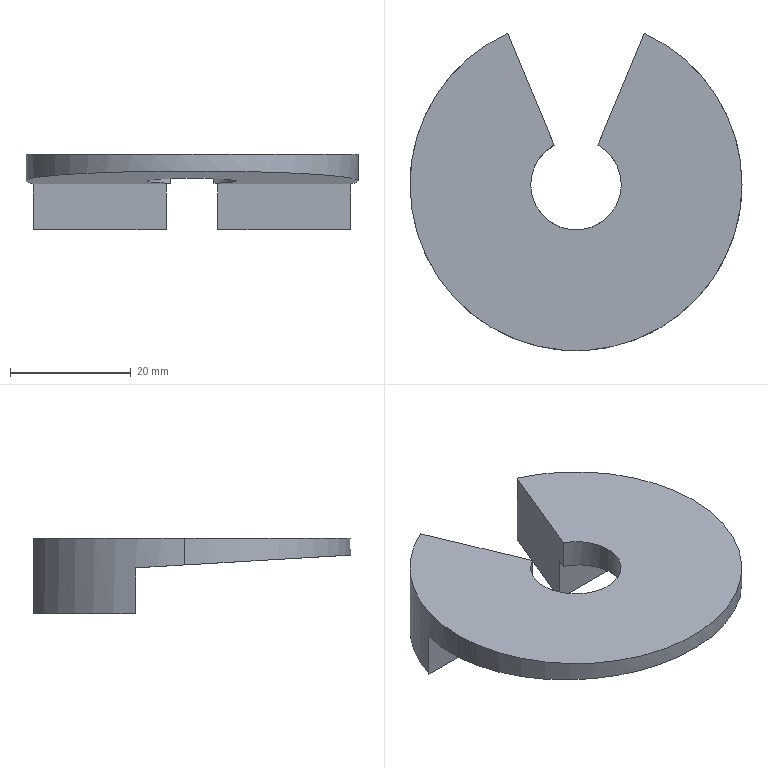Part | SolidWorks | features BaseBody 1, HoleWzd 1 | 1 solid | 22 faces | box 55 x 52.573 x 12.5 mm | volume 11112 mm3 | cylinder 10 | plane 8 | cone 4 | commonest cylinder face diameters 3.3 x4 15 x3 55 x3
STEP:
#1=CARTESIAN_POINT('',(17.65,-3.,161.));
#2=VERTEX_POINT('',#1);
#3=CARTESIAN_POINT('',(14.35,-3.,161.));
#4=VERTEX_POINT('',#3);
#5=CARTESIAN_POINT('',(16.,-3.,161.));
#6=DIRECTION('',(0.,0.,-1.));
#7=DIRECTION('',(-1.,0.,0.));
#8=AXIS2_PLACEMENT_3D('',#5,#6,#7);
#9=CIRCLE('',#8,1.65);
#10=EDGE_CURVE('',#2,#4,#9,.T.);
#11=ORIENTED_EDGE('',*,*,#10,.F.);
#12=CARTESIAN_POINT('',(17.65,-3.,154.));
#13=VERTEX_POINT('',#12);
#14=CARTESIAN_POINT('',(17.65,-3.,154.));
#15=DIRECTION('',(0.,0.,-1.));
#16=VECTOR('',#15,1000.);
#17=LINE('',#14,#16);
#18=EDGE_CURVE('',#2,#13,#17,.T.);
#19=ORIENTED_EDGE('',*,*,#18,.T.);
#20=CARTESIAN_POINT('',(14.35,-3.,154.));
#21=VERTEX_POINT('',#20);
#22=CARTESIAN_POINT('',(16.,-3.,154.));
#23=DIRECTION('',(0.,0.,-1.));
#24=DIRECTION('',(-1.,0.,0.));
#25=AXIS2_PLACEMENT_3D('',#22,#23,#24);
#26=CIRCLE('',#25,1.65);
#27=EDGE_CURVE('',#13,#21,#26,.T.);
#28=ORIENTED_EDGE('',*,*,#27,.T.);
#29=CARTESIAN_POINT('',(14.35,-3.,154.));
#30=DIRECTION('',(0.,0.,-1.));
#31=VECTOR('',#30,1000.);
#32=LINE('',#29,#31);
#33=EDGE_CURVE('',#4,#21,#32,.T.);
#34=ORIENTED_EDGE('',*,*,#33,.F.);
#35=EDGE_LOOP('',(#11,#19,#28,#34));
#36=FACE_OUTER_BOUND('',#35,.T.);
#37=CARTESIAN_POINT('',(16.,-3.,154.));
#38=DIRECTION('',(0.,0.,-1.));
#39=DIRECTION('',(-1.,0.,0.));
#40=AXIS2_PLACEMENT_3D('',#37,#38,#39);
#41=CYLINDRICAL_SURFACE('',#40,1.65);
#42=ADVANCED_FACE('',(#36),#41,.F.);
#43=CARTESIAN_POINT('',(16.,-3.,161.991));
#44=VERTEX_POINT('',#43);
#45=CARTESIAN_POINT('',(14.35,-3.,161.));
#46=DIRECTION('',(-0.8572,0.,-0.515));
#47=VECTOR('',#46,1000.);
#48=LINE('',#45,#47);
#49=EDGE_CURVE('',#44,#4,#48,.T.);
#50=ORIENTED_EDGE('',*,*,#49,.F.);
#51=CARTESIAN_POINT('',(17.65,-3.,161.));
#52=DIRECTION('',(0.8572,0.,-0.515));
#53=VECTOR('',#52,1000.);
#54=LINE('',#51,#53);
#55=EDGE_CURVE('',#44,#2,#54,.T.);
#56=ORIENTED_EDGE('',*,*,#55,.T.);
#57=ORIENTED_EDGE('',*,*,#10,.T.);
#58=EDGE_LOOP('',(#50,#56,#57));
#59=FACE_OUTER_BOUND('',#58,.T.);
#60=CARTESIAN_POINT('',(16.,-3.,161.));
#61=DIRECTION('',(0.,0.,-1.));
#62=DIRECTION('',(-1.,0.,0.));
#63=AXIS2_PLACEMENT_3D('',#60,#61,#62);
#64=CONICAL_SURFACE('',#63,1.65,1.03);
#65=ADVANCED_FACE('',(#59),#64,.F.);
#66=CARTESIAN_POINT('',(-14.35,-3.,161.));
#67=VERTEX_POINT('',#66);
#68=CARTESIAN_POINT('',(-17.65,-3.,161.));
#69=VERTEX_POINT('',#68);
#70=CARTESIAN_POINT('',(-16.,-3.,161.));
#71=DIRECTION('',(0.,0.,-1.));
#72=DIRECTION('',(-1.,0.,0.));
#73=AXIS2_PLACEMENT_3D('',#70,#71,#72);
#74=CIRCLE('',#73,1.65);
#75=EDGE_CURVE('',#67,#69,#74,.T.);
#76=ORIENTED_EDGE('',*,*,#75,.F.);
#77=CARTESIAN_POINT('',(-14.35,-3.,154.));
#78=VERTEX_POINT('',#77);
#79=CARTESIAN_POINT('',(-14.35,-3.,154.));
#80=DIRECTION('',(0.,0.,-1.));
#81=VECTOR('',#80,1000.);
#82=LINE('',#79,#81);
#83=EDGE_CURVE('',#67,#78,#82,.T.);
#84=ORIENTED_EDGE('',*,*,#83,.T.);
#85=CARTESIAN_POINT('',(-17.65,-3.,154.));
#86=VERTEX_POINT('',#85);
#87=CARTESIAN_POINT('',(-16.,-3.,154.));
#88=DIRECTION('',(0.,0.,-1.));
#89=DIRECTION('',(-1.,0.,0.));
#90=AXIS2_PLACEMENT_3D('',#87,#88,#89);
#91=CIRCLE('',#90,1.65);
#92=EDGE_CURVE('',#78,#86,#91,.T.);
#93=ORIENTED_EDGE('',*,*,#92,.T.);
#94=CARTESIAN_POINT('',(-17.65,-3.,154.));
#95=DIRECTION('',(0.,0.,-1.));
#96=VECTOR('',#95,1000.);
#97=LINE('',#94,#96);
#98=EDGE_CURVE('',#69,#86,#97,.T.);
#99=ORIENTED_EDGE('',*,*,#98,.F.);
#100=EDGE_LOOP('',(#76,#84,#93,#99));
#101=FACE_OUTER_BOUND('',#100,.T.);
#102=CARTESIAN_POINT('',(-16.,-3.,154.));
#103=DIRECTION('',(0.,0.,-1.));
#104=DIRECTION('',(-1.,0.,0.));
#105=AXIS2_PLACEMENT_3D('',#102,#103,#104);
#106=CYLINDRICAL_SURFACE('',#105,1.65);
#107=ADVANCED_FACE('',(#101),#106,.F.);
#108=CARTESIAN_POINT('',(-16.,-3.,161.991));
#109=VERTEX_POINT('',#108);
#110=CARTESIAN_POINT('',(-17.65,-3.,161.));
#111=DIRECTION('',(-0.8572,0.,-0.515));
#112=VECTOR('',#111,1000.);
#113=LINE('',#110,#112);
#114=EDGE_CURVE('',#109,#69,#113,.T.);
#115=ORIENTED_EDGE('',*,*,#114,.F.);
#116=CARTESIAN_POINT('',(-14.35,-3.,161.));
#117=DIRECTION('',(0.8572,0.,-0.515));
#118=VECTOR('',#117,1000.);
#119=LINE('',#116,#118);
#120=EDGE_CURVE('',#109,#67,#119,.T.);
#121=ORIENTED_EDGE('',*,*,#120,.T.);
#122=ORIENTED_EDGE('',*,*,#75,.T.);
#123=EDGE_LOOP('',(#115,#121,#122));
#124=FACE_OUTER_BOUND('',#123,.T.);
#125=CARTESIAN_POINT('',(-16.,-3.,161.));
#126=DIRECTION('',(0.,0.,-1.));
#127=DIRECTION('',(-1.,0.,0.));
#128=AXIS2_PLACEMENT_3D('',#125,#126,#127);
#129=CONICAL_SURFACE('',#128,1.65,1.03);
#130=ADVANCED_FACE('',(#124),#129,.F.);
#131=CARTESIAN_POINT('',(7.5,-17.,166.5));
#132=VERTEX_POINT('',#131);
#133=CARTESIAN_POINT('',(-7.5,-17.,166.5));
#134=VERTEX_POINT('',#133);
#135=CARTESIAN_POINT('',(0.,-17.,166.5));
#136=DIRECTION('',(0.,0.,-1.));
#137=DIRECTION('',(-1.,0.,0.));
#138=AXIS2_PLACEMENT_3D('',#135,#136,#137);
#139=CIRCLE('',#138,7.5);
#140=EDGE_CURVE('',#132,#134,#139,.T.);
#141=ORIENTED_EDGE('',*,*,#140,.F.);
#142=CARTESIAN_POINT('',(7.5,-17.,162.084));
#143=VERTEX_POINT('',#142);
#144=CARTESIAN_POINT('',(7.5,-17.,166.5));
#145=DIRECTION('',(0.,0.,-1.));
#146=VECTOR('',#145,1000.);
#147=LINE('',#144,#146);
#148=EDGE_CURVE('',#132,#143,#147,.T.);
#149=ORIENTED_EDGE('',*,*,#148,.T.);
#150=CARTESIAN_POINT('',(-7.5,-17.,162.084));
#151=VERTEX_POINT('',#150);
#152=CARTESIAN_POINT('',(-7.5,-17.,162.084));
#153=CARTESIAN_POINT('',(-7.5,-32.,162.973));
#154=CARTESIAN_POINT('',(7.5,-32.,162.973));
#155=CARTESIAN_POINT('',(7.5,-17.,162.084));
#156=(BOUNDED_CURVE()B_SPLINE_CURVE(3,(#152,#153,#154,#155),.UNSPECIFIED.,.F.,.F.)B_SPLINE_CURVE_WITH_KNOTS((4,4),(1.571,4.712),.UNSPECIFIED.)CURVE()GEOMETRIC_REPRESENTATION_ITEM()RATIONAL_B_SPLINE_CURVE((1.,0.3333,0.3333,1.))REPRESENTATION_ITEM(''));
#157=EDGE_CURVE('',#151,#143,#156,.T.);
#158=ORIENTED_EDGE('',*,*,#157,.F.);
#159=CARTESIAN_POINT('',(-7.5,-17.,166.5));
#160=DIRECTION('',(0.,0.,-1.));
#161=VECTOR('',#160,1000.);
#162=LINE('',#159,#161);
#163=EDGE_CURVE('',#134,#151,#162,.T.);
#164=ORIENTED_EDGE('',*,*,#163,.F.);
#165=EDGE_LOOP('',(#141,#149,#158,#164));
#166=FACE_OUTER_BOUND('',#165,.T.);
#167=CARTESIAN_POINT('',(0.,-17.,166.5));
#168=DIRECTION('',(0.,0.,-1.));
#169=DIRECTION('',(-1.,0.,0.));
#170=AXIS2_PLACEMENT_3D('',#167,#168,#169);
#171=CYLINDRICAL_SURFACE('',#170,7.5);
#172=ADVANCED_FACE('',(#166),#171,.F.);
#173=CARTESIAN_POINT('',(-3.629,-10.437,166.5));
#174=VERTEX_POINT('',#173);
#175=CARTESIAN_POINT('',(0.,-17.,166.5));
#176=DIRECTION('',(0.,0.,-1.));
#177=DIRECTION('',(-1.,0.,0.));
#178=AXIS2_PLACEMENT_3D('',#175,#176,#177);
#179=CIRCLE('',#178,7.5);
#180=EDGE_CURVE('',#134,#174,#179,.T.);
#181=ORIENTED_EDGE('',*,*,#180,.F.);
#182=ORIENTED_EDGE('',*,*,#163,.T.);
#183=CARTESIAN_POINT('',(-3.629,-10.437,161.695));
#184=VERTEX_POINT('',#183);
#185=CARTESIAN_POINT('',(-3.629,-10.437,161.695));
#186=CARTESIAN_POINT('',(-6.078,-11.791,161.775));
#187=CARTESIAN_POINT('',(-7.5,-14.201,161.918));
#188=CARTESIAN_POINT('',(-7.5,-17.,162.084));
#189=(BOUNDED_CURVE()B_SPLINE_CURVE(3,(#185,#186,#187,#188),.UNSPECIFIED.,.F.,.F.)B_SPLINE_CURVE_WITH_KNOTS((4,4),(0.5051,1.571),.UNSPECIFIED.)CURVE()GEOMETRIC_REPRESENTATION_ITEM()RATIONAL_B_SPLINE_CURVE((1.,0.9076,0.9076,1.))REPRESENTATION_ITEM(''));
#190=EDGE_CURVE('',#184,#151,#189,.T.);
#191=ORIENTED_EDGE('',*,*,#190,.F.);
#192=CARTESIAN_POINT('',(-3.629,-10.437,166.5));
#193=DIRECTION('',(0.,0.,1.));
#194=VECTOR('',#193,1000.);
#195=LINE('',#192,#194);
#196=EDGE_CURVE('',#184,#174,#195,.T.);
#197=ORIENTED_EDGE('',*,*,#196,.T.);
#198=EDGE_LOOP('',(#181,#182,#191,#197));
#199=FACE_OUTER_BOUND('',#198,.T.);
#200=CARTESIAN_POINT('',(0.,-17.,166.5));
#201=DIRECTION('',(0.,0.,-1.));
#202=DIRECTION('',(-1.,0.,0.));
#203=AXIS2_PLACEMENT_3D('',#200,#201,#202);
#204=CYLINDRICAL_SURFACE('',#203,7.5);
#205=ADVANCED_FACE('',(#199),#204,.F.);
#206=CARTESIAN_POINT('',(27.5,-17.,166.5));
#207=VERTEX_POINT('',#206);
#208=CARTESIAN_POINT('',(11.296,8.073,166.5));
#209=VERTEX_POINT('',#208);
#210=CARTESIAN_POINT('',(0.,-17.,166.5));
#211=DIRECTION('',(0.,0.,1.));
#212=DIRECTION('',(-1.,0.,0.));
#213=AXIS2_PLACEMENT_3D('',#210,#211,#212);
#214=CIRCLE('',#213,27.5);
#215=EDGE_CURVE('',#207,#209,#214,.T.);
#216=ORIENTED_EDGE('',*,*,#215,.F.);
#217=CARTESIAN_POINT('',(27.5,-17.,162.084));
#218=VERTEX_POINT('',#217);
#219=CARTESIAN_POINT('',(27.5,-17.,166.5));
#220=DIRECTION('',(0.,0.,-1.));
#221=VECTOR('',#220,1000.);
#222=LINE('',#219,#221);
#223=EDGE_CURVE('',#207,#218,#222,.T.);
#224=ORIENTED_EDGE('',*,*,#223,.T.);
#225=CARTESIAN_POINT('',(26.269,-8.864,161.602));
#226=VERTEX_POINT('',#225);
#227=CARTESIAN_POINT('',(27.5,-17.,162.084));
#228=CARTESIAN_POINT('',(27.5,-14.237,161.92));
#229=CARTESIAN_POINT('',(27.087,-11.504,161.758));
#230=CARTESIAN_POINT('',(26.269,-8.864,161.602));
#231=(BOUNDED_CURVE()B_SPLINE_CURVE(3,(#227,#228,#229,#230),.UNSPECIFIED.,.F.,.F.)B_SPLINE_CURVE_WITH_KNOTS((4,4),(4.712,5.013),.UNSPECIFIED.)CURVE()GEOMETRIC_REPRESENTATION_ITEM()RATIONAL_B_SPLINE_CURVE((1.,0.9925,0.9925,1.))REPRESENTATION_ITEM(''));
#232=EDGE_CURVE('',#218,#226,#231,.T.);
#233=ORIENTED_EDGE('',*,*,#232,.T.);
#234=CARTESIAN_POINT('',(26.269,-8.864,154.));
#235=VERTEX_POINT('',#234);
#236=CARTESIAN_POINT('',(26.269,-8.864,166.5));
#237=DIRECTION('',(0.,0.,-1.));
#238=VECTOR('',#237,1000.);
#239=LINE('',#236,#238);
#240=EDGE_CURVE('',#226,#235,#239,.T.);
#241=ORIENTED_EDGE('',*,*,#240,.T.);
#242=CARTESIAN_POINT('',(11.296,8.073,154.));
#243=VERTEX_POINT('',#242);
#244=CARTESIAN_POINT('',(0.,-17.,154.));
#245=DIRECTION('',(0.,0.,1.));
#246=DIRECTION('',(-1.,0.,0.));
#247=AXIS2_PLACEMENT_3D('',#244,#245,#246);
#248=CIRCLE('',#247,27.5);
#249=EDGE_CURVE('',#235,#243,#248,.T.);
#250=ORIENTED_EDGE('',*,*,#249,.T.);
#251=CARTESIAN_POINT('',(11.296,8.073,166.5));
#252=DIRECTION('',(0.,0.,1.));
#253=VECTOR('',#252,1000.);
#254=LINE('',#251,#253);
#255=EDGE_CURVE('',#243,#209,#254,.T.);
#256=ORIENTED_EDGE('',*,*,#255,.T.);
#257=EDGE_LOOP('',(#216,#224,#233,#241,#250,#256));
#258=FACE_OUTER_BOUND('',#257,.T.);
#259=CARTESIAN_POINT('',(0.,-17.,166.5));
#260=DIRECTION('',(0.,0.,-1.));
#261=DIRECTION('',(-1.,0.,0.));
#262=AXIS2_PLACEMENT_3D('',#259,#260,#261);
#263=CYLINDRICAL_SURFACE('',#262,27.5);
#264=ADVANCED_FACE('',(#258),#263,.T.);
#265=ORIENTED_EDGE('',*,*,#223,.F.);
#266=CARTESIAN_POINT('',(-27.5,-17.,166.5));
#267=VERTEX_POINT('',#266);
#268=CARTESIAN_POINT('',(0.,-17.,166.5));
#269=DIRECTION('',(0.,0.,1.));
#270=DIRECTION('',(-1.,0.,0.));
#271=AXIS2_PLACEMENT_3D('',#268,#269,#270);
#272=CIRCLE('',#271,27.5);
#273=EDGE_CURVE('',#267,#207,#272,.T.);
#274=ORIENTED_EDGE('',*,*,#273,.F.);
#275=CARTESIAN_POINT('',(-27.5,-17.,162.084));
#276=VERTEX_POINT('',#275);
#277=CARTESIAN_POINT('',(-27.5,-17.,166.5));
#278=DIRECTION('',(0.,0.,-1.));
#279=VECTOR('',#278,1000.);
#280=LINE('',#277,#279);
#281=EDGE_CURVE('',#267,#276,#280,.T.);
#282=ORIENTED_EDGE('',*,*,#281,.T.);
#283=CARTESIAN_POINT('',(-27.5,-17.,162.084));
#284=CARTESIAN_POINT('',(-27.5,-72.,165.343));
#285=CARTESIAN_POINT('',(27.5,-72.,165.343));
#286=CARTESIAN_POINT('',(27.5,-17.,162.084));
#287=(BOUNDED_CURVE()B_SPLINE_CURVE(3,(#283,#284,#285,#286),.UNSPECIFIED.,.F.,.F.)B_SPLINE_CURVE_WITH_KNOTS((4,4),(1.571,4.712),.UNSPECIFIED.)CURVE()GEOMETRIC_REPRESENTATION_ITEM()RATIONAL_B_SPLINE_CURVE((1.,0.3333,0.3333,1.))REPRESENTATION_ITEM(''));
#288=EDGE_CURVE('',#276,#218,#287,.T.);
#289=ORIENTED_EDGE('',*,*,#288,.T.);
#290=EDGE_LOOP('',(#265,#274,#282,#289));
#291=FACE_OUTER_BOUND('',#290,.T.);
#292=CARTESIAN_POINT('',(0.,-17.,166.5));
#293=DIRECTION('',(0.,0.,-1.));
#294=DIRECTION('',(-1.,0.,0.));
#295=AXIS2_PLACEMENT_3D('',#292,#293,#294);
#296=CYLINDRICAL_SURFACE('',#295,27.5);
#297=ADVANCED_FACE('',(#291),#296,.T.);
#298=CARTESIAN_POINT('',(3.629,-10.437,166.5));
#299=VERTEX_POINT('',#298);
#300=CARTESIAN_POINT('',(0.,-17.,166.5));
#301=DIRECTION('',(0.,0.,-1.));
#302=DIRECTION('',(-1.,0.,0.));
#303=AXIS2_PLACEMENT_3D('',#300,#301,#302);
#304=CIRCLE('',#303,7.5);
#305=EDGE_CURVE('',#299,#132,#304,.T.);
#306=ORIENTED_EDGE('',*,*,#305,.T.);
#307=ORIENTED_EDGE('',*,*,#140,.T.);
#308=ORIENTED_EDGE('',*,*,#180,.T.);
#309=CARTESIAN_POINT('',(-11.296,8.073,166.5));
#310=VERTEX_POINT('',#309);
#311=CARTESIAN_POINT('',(-3.629,-10.437,166.5));
#312=DIRECTION('',(-0.3827,0.9239,0.));
#313=VECTOR('',#312,1000.);
#314=LINE('',#311,#313);
#315=EDGE_CURVE('',#174,#310,#314,.T.);
#316=ORIENTED_EDGE('',*,*,#315,.T.);
#317=CARTESIAN_POINT('',(0.,-17.,166.5));
#318=DIRECTION('',(0.,0.,1.));
#319=DIRECTION('',(-1.,0.,0.));
#320=AXIS2_PLACEMENT_3D('',#317,#318,#319);
#321=CIRCLE('',#320,27.5);
#322=EDGE_CURVE('',#310,#267,#321,.T.);
#323=ORIENTED_EDGE('',*,*,#322,.T.);
#324=ORIENTED_EDGE('',*,*,#273,.T.);
#325=ORIENTED_EDGE('',*,*,#215,.T.);
#326=CARTESIAN_POINT('',(11.296,8.073,166.5));
#327=DIRECTION('',(-0.3827,-0.9239,0.));
#328=VECTOR('',#327,1000.);
#329=LINE('',#326,#328);
#330=EDGE_CURVE('',#209,#299,#329,.T.);
#331=ORIENTED_EDGE('',*,*,#330,.T.);
#332=EDGE_LOOP('',(#306,#307,#308,#316,#323,#324,#325,#331));
#333=FACE_OUTER_BOUND('',#332,.T.);
#334=CARTESIAN_POINT('',(0.,-17.,166.5));
#335=DIRECTION('',(0.,0.,1.));
#336=DIRECTION('',(1.,0.,0.));
#337=AXIS2_PLACEMENT_3D('',#334,#335,#336);
#338=PLANE('',#337);
#339=ADVANCED_FACE('',(#333),#338,.T.);
#340=CARTESIAN_POINT('',(-4.28,-8.864,161.602));
#341=VERTEX_POINT('',#340);
#342=CARTESIAN_POINT('',(-3.629,-10.437,161.695));
#343=DIRECTION('',(-0.3821,0.9225,-0.05467));
#344=VECTOR('',#343,1000.);
#345=LINE('',#342,#344);
#346=EDGE_CURVE('',#184,#341,#345,.T.);
#347=ORIENTED_EDGE('',*,*,#346,.T.);
#348=CARTESIAN_POINT('',(-4.28,-8.864,154.));
#349=VERTEX_POINT('',#348);
#350=CARTESIAN_POINT('',(-4.28,-8.864,166.5));
#351=DIRECTION('',(0.,0.,1.));
#352=VECTOR('',#351,1000.);
#353=LINE('',#350,#352);
#354=EDGE_CURVE('',#349,#341,#353,.T.);
#355=ORIENTED_EDGE('',*,*,#354,.F.);
#356=CARTESIAN_POINT('',(-11.296,8.073,154.));
#357=VERTEX_POINT('',#356);
#358=CARTESIAN_POINT('',(-11.296,8.073,154.));
#359=DIRECTION('',(0.3827,-0.9239,0.));
#360=VECTOR('',#359,1000.);
#361=LINE('',#358,#360);
#362=EDGE_CURVE('',#357,#349,#361,.T.);
#363=ORIENTED_EDGE('',*,*,#362,.F.);
#364=CARTESIAN_POINT('',(-11.296,8.073,166.5));
#365=DIRECTION('',(0.,0.,-1.));
#366=VECTOR('',#365,1000.);
#367=LINE('',#364,#366);
#368=EDGE_CURVE('',#310,#357,#367,.T.);
#369=ORIENTED_EDGE('',*,*,#368,.F.);
#370=ORIENTED_EDGE('',*,*,#315,.F.);
#371=ORIENTED_EDGE('',*,*,#196,.F.);
#372=EDGE_LOOP('',(#347,#355,#363,#369,#370,#371));
#373=FACE_OUTER_BOUND('',#372,.T.);
#374=CARTESIAN_POINT('',(-11.296,8.073,166.5));
#375=DIRECTION('',(-0.9239,-0.3827,0.));
#376=DIRECTION('',(0.3827,-0.9239,0.));
#377=AXIS2_PLACEMENT_3D('',#374,#375,#376);
#378=PLANE('',#377);
#379=ADVANCED_FACE('',(#373),#378,.F.);
#380=ORIENTED_EDGE('',*,*,#148,.F.);
#381=ORIENTED_EDGE('',*,*,#305,.F.);
#382=CARTESIAN_POINT('',(3.629,-10.437,161.695));
#383=VERTEX_POINT('',#382);
#384=CARTESIAN_POINT('',(3.629,-10.437,166.5));
#385=DIRECTION('',(0.,0.,1.));
#386=VECTOR('',#385,1000.);
#387=LINE('',#384,#386);
#388=EDGE_CURVE('',#383,#299,#387,.T.);
#389=ORIENTED_EDGE('',*,*,#388,.F.);
#390=CARTESIAN_POINT('',(7.5,-17.,162.084));
#391=CARTESIAN_POINT('',(7.5,-14.201,161.918));
#392=CARTESIAN_POINT('',(6.078,-11.791,161.775));
#393=CARTESIAN_POINT('',(3.629,-10.437,161.695));
#394=(BOUNDED_CURVE()B_SPLINE_CURVE(3,(#390,#391,#392,#393),.UNSPECIFIED.,.F.,.T.)B_SPLINE_CURVE_WITH_KNOTS((4,4),(4.712,5.778),.UNSPECIFIED.)CURVE()GEOMETRIC_REPRESENTATION_ITEM()RATIONAL_B_SPLINE_CURVE((1.,0.9076,0.9076,1.))REPRESENTATION_ITEM(''));
#395=EDGE_CURVE('',#143,#383,#394,.T.);
#396=ORIENTED_EDGE('',*,*,#395,.F.);
#397=EDGE_LOOP('',(#380,#381,#389,#396));
#398=FACE_OUTER_BOUND('',#397,.T.);
#399=CARTESIAN_POINT('',(0.,-17.,166.5));
#400=DIRECTION('',(0.,0.,-1.));
#401=DIRECTION('',(-1.,0.,0.));
#402=AXIS2_PLACEMENT_3D('',#399,#400,#401);
#403=CYLINDRICAL_SURFACE('',#402,7.5);
#404=ADVANCED_FACE('',(#398),#403,.F.);
#405=CARTESIAN_POINT('',(4.28,-8.864,161.602));
#406=VERTEX_POINT('',#405);
#407=CARTESIAN_POINT('',(3.629,-10.437,161.695));
#408=DIRECTION('',(0.3821,0.9225,-0.05467));
#409=VECTOR('',#408,1000.);
#410=LINE('',#407,#409);
#411=EDGE_CURVE('',#383,#406,#410,.T.);
#412=ORIENTED_EDGE('',*,*,#411,.F.);
#413=ORIENTED_EDGE('',*,*,#388,.T.);
#414=ORIENTED_EDGE('',*,*,#330,.F.);
#415=ORIENTED_EDGE('',*,*,#255,.F.);
#416=CARTESIAN_POINT('',(4.28,-8.864,154.));
#417=VERTEX_POINT('',#416);
#418=CARTESIAN_POINT('',(11.296,8.073,154.));
#419=DIRECTION('',(0.3827,0.9239,0.));
#420=VECTOR('',#419,1000.);
#421=LINE('',#418,#420);
#422=EDGE_CURVE('',#417,#243,#421,.T.);
#423=ORIENTED_EDGE('',*,*,#422,.F.);
#424=CARTESIAN_POINT('',(4.28,-8.864,166.5));
#425=DIRECTION('',(0.,0.,-1.));
#426=VECTOR('',#425,1000.);
#427=LINE('',#424,#426);
#428=EDGE_CURVE('',#406,#417,#427,.T.);
#429=ORIENTED_EDGE('',*,*,#428,.F.);
#430=EDGE_LOOP('',(#412,#413,#414,#415,#423,#429));
#431=FACE_OUTER_BOUND('',#430,.T.);
#432=CARTESIAN_POINT('',(11.296,8.073,166.5));
#433=DIRECTION('',(0.9239,-0.3827,0.));
#434=DIRECTION('',(0.3827,0.9239,0.));
#435=AXIS2_PLACEMENT_3D('',#432,#433,#434);
#436=PLANE('',#435);
#437=ADVANCED_FACE('',(#431),#436,.F.);
#438=ORIENTED_EDGE('',*,*,#281,.F.);
#439=ORIENTED_EDGE('',*,*,#322,.F.);
#440=ORIENTED_EDGE('',*,*,#368,.T.);
#441=CARTESIAN_POINT('',(-26.269,-8.864,154.));
#442=VERTEX_POINT('',#441);
#443=CARTESIAN_POINT('',(0.,-17.,154.));
#444=DIRECTION('',(0.,0.,1.));
#445=DIRECTION('',(-1.,0.,0.));
#446=AXIS2_PLACEMENT_3D('',#443,#444,#445);
#447=CIRCLE('',#446,27.5);
#448=EDGE_CURVE('',#357,#442,#447,.T.);
#449=ORIENTED_EDGE('',*,*,#448,.T.);
#450=CARTESIAN_POINT('',(-26.269,-8.864,161.602));
#451=VERTEX_POINT('',#450);
#452=CARTESIAN_POINT('',(-26.269,-8.864,166.5));
#453=DIRECTION('',(0.,0.,1.));
#454=VECTOR('',#453,1000.);
#455=LINE('',#452,#454);
#456=EDGE_CURVE('',#442,#451,#455,.T.);
#457=ORIENTED_EDGE('',*,*,#456,.T.);
#458=CARTESIAN_POINT('',(-26.269,-8.864,161.602));
#459=CARTESIAN_POINT('',(-27.087,-11.504,161.758));
#460=CARTESIAN_POINT('',(-27.5,-14.237,161.92));
#461=CARTESIAN_POINT('',(-27.5,-17.,162.084));
#462=(BOUNDED_CURVE()B_SPLINE_CURVE(3,(#458,#459,#460,#461),.UNSPECIFIED.,.F.,.F.)B_SPLINE_CURVE_WITH_KNOTS((4,4),(1.27,1.571),.UNSPECIFIED.)CURVE()GEOMETRIC_REPRESENTATION_ITEM()RATIONAL_B_SPLINE_CURVE((1.,0.9925,0.9925,1.))REPRESENTATION_ITEM(''));
#463=EDGE_CURVE('',#451,#276,#462,.T.);
#464=ORIENTED_EDGE('',*,*,#463,.T.);
#465=EDGE_LOOP('',(#438,#439,#440,#449,#457,#464));
#466=FACE_OUTER_BOUND('',#465,.T.);
#467=CARTESIAN_POINT('',(0.,-17.,166.5));
#468=DIRECTION('',(0.,0.,-1.));
#469=DIRECTION('',(-1.,0.,0.));
#470=AXIS2_PLACEMENT_3D('',#467,#468,#469);
#471=CYLINDRICAL_SURFACE('',#470,27.5);
#472=ADVANCED_FACE('',(#466),#471,.T.);
#473=ORIENTED_EDGE('',*,*,#354,.T.);
#474=CARTESIAN_POINT('',(-30.,-8.864,161.602));
#475=DIRECTION('',(1.,0.,0.));
#476=VECTOR('',#475,1000.);
#477=LINE('',#474,#476);
#478=EDGE_CURVE('',#451,#341,#477,.T.);
#479=ORIENTED_EDGE('',*,*,#478,.F.);
#480=ORIENTED_EDGE('',*,*,#456,.F.);
#481=CARTESIAN_POINT('',(-30.,-8.864,154.));
#482=DIRECTION('',(-1.,0.,0.));
#483=VECTOR('',#482,1000.);
#484=LINE('',#481,#483);
#485=EDGE_CURVE('',#349,#442,#484,.T.);
#486=ORIENTED_EDGE('',*,*,#485,.F.);
#487=EDGE_LOOP('',(#473,#479,#480,#486));
#488=FACE_OUTER_BOUND('',#487,.T.);
#489=CARTESIAN_POINT('',(-30.,-8.864,154.));
#490=DIRECTION('',(0.,1.,0.));
#491=DIRECTION('',(0.,0.,1.));
#492=AXIS2_PLACEMENT_3D('',#489,#490,#491);
#493=PLANE('',#492);
#494=ADVANCED_FACE('',(#488),#493,.F.);
#495=CARTESIAN_POINT('',(-16.,-3.,154.));
#496=DIRECTION('',(0.,0.,-1.));
#497=DIRECTION('',(-1.,0.,0.));
#498=AXIS2_PLACEMENT_3D('',#495,#496,#497);
#499=CIRCLE('',#498,1.65);
#500=EDGE_CURVE('',#86,#78,#499,.T.);
#501=ORIENTED_EDGE('',*,*,#500,.F.);
#502=ORIENTED_EDGE('',*,*,#92,.F.);
#503=EDGE_LOOP('',(#501,#502));
#504=FACE_BOUND('',#503,.T.);
#505=ORIENTED_EDGE('',*,*,#485,.T.);
#506=ORIENTED_EDGE('',*,*,#448,.F.);
#507=ORIENTED_EDGE('',*,*,#362,.T.);
#508=EDGE_LOOP('',(#505,#506,#507));
#509=FACE_OUTER_BOUND('',#508,.T.);
#510=CARTESIAN_POINT('',(0.,-17.,154.));
#511=DIRECTION('',(0.,0.,1.));
#512=DIRECTION('',(1.,0.,0.));
#513=AXIS2_PLACEMENT_3D('',#510,#511,#512);
#514=PLANE('',#513);
#515=ADVANCED_FACE('',(#504,#509),#514,.F.);
#516=ORIENTED_EDGE('',*,*,#346,.F.);
#517=ORIENTED_EDGE('',*,*,#190,.T.);
#518=ORIENTED_EDGE('',*,*,#157,.T.);
#519=ORIENTED_EDGE('',*,*,#395,.T.);
#520=ORIENTED_EDGE('',*,*,#411,.T.);
#521=CARTESIAN_POINT('',(-30.,-8.864,161.602));
#522=DIRECTION('',(-1.,0.,0.));
#523=VECTOR('',#522,1000.);
#524=LINE('',#521,#523);
#525=EDGE_CURVE('',#226,#406,#524,.T.);
#526=ORIENTED_EDGE('',*,*,#525,.F.);
#527=ORIENTED_EDGE('',*,*,#232,.F.);
#528=ORIENTED_EDGE('',*,*,#288,.F.);
#529=ORIENTED_EDGE('',*,*,#463,.F.);
#530=ORIENTED_EDGE('',*,*,#478,.T.);
#531=EDGE_LOOP('',(#516,#517,#518,#519,#520,#526,#527,#528,#529,#530));
#532=FACE_OUTER_BOUND('',#531,.T.);
#533=CARTESIAN_POINT('',(-30.,-8.864,161.602));
#534=DIRECTION('',(0.,0.05916,0.9982));
#535=DIRECTION('',(0.,-0.9982,0.05916));
#536=AXIS2_PLACEMENT_3D('',#533,#534,#535);
#537=PLANE('',#536);
#538=ADVANCED_FACE('',(#532),#537,.F.);
#539=ORIENTED_EDGE('',*,*,#428,.T.);
#540=CARTESIAN_POINT('',(-30.,-8.864,154.));
#541=DIRECTION('',(-1.,0.,0.));
#542=VECTOR('',#541,1000.);
#543=LINE('',#540,#542);
#544=EDGE_CURVE('',#235,#417,#543,.T.);
#545=ORIENTED_EDGE('',*,*,#544,.F.);
#546=ORIENTED_EDGE('',*,*,#240,.F.);
#547=ORIENTED_EDGE('',*,*,#525,.T.);
#548=EDGE_LOOP('',(#539,#545,#546,#547));
#549=FACE_OUTER_BOUND('',#548,.T.);
#550=CARTESIAN_POINT('',(-30.,-8.864,154.));
#551=DIRECTION('',(0.,1.,0.));
#552=DIRECTION('',(0.,0.,1.));
#553=AXIS2_PLACEMENT_3D('',#550,#551,#552);
#554=PLANE('',#553);
#555=ADVANCED_FACE('',(#549),#554,.F.);
#556=CARTESIAN_POINT('',(16.,-3.,154.));
#557=DIRECTION('',(0.,0.,-1.));
#558=DIRECTION('',(-1.,0.,0.));
#559=AXIS2_PLACEMENT_3D('',#556,#557,#558);
#560=CIRCLE('',#559,1.65);
#561=EDGE_CURVE('',#21,#13,#560,.T.);
#562=ORIENTED_EDGE('',*,*,#561,.F.);
#563=ORIENTED_EDGE('',*,*,#27,.F.);
#564=EDGE_LOOP('',(#562,#563));
#565=FACE_BOUND('',#564,.T.);
#566=ORIENTED_EDGE('',*,*,#544,.T.);
#567=ORIENTED_EDGE('',*,*,#422,.T.);
#568=ORIENTED_EDGE('',*,*,#249,.F.);
#569=EDGE_LOOP('',(#566,#567,#568));
#570=FACE_OUTER_BOUND('',#569,.T.);
#571=CARTESIAN_POINT('',(0.,-17.,154.));
#572=DIRECTION('',(0.,0.,1.));
#573=DIRECTION('',(1.,0.,0.));
#574=AXIS2_PLACEMENT_3D('',#571,#572,#573);
#575=PLANE('',#574);
#576=ADVANCED_FACE('',(#565,#570),#575,.F.);
#577=ORIENTED_EDGE('',*,*,#120,.F.);
#578=ORIENTED_EDGE('',*,*,#114,.T.);
#579=CARTESIAN_POINT('',(-16.,-3.,161.));
#580=DIRECTION('',(0.,0.,-1.));
#581=DIRECTION('',(-1.,0.,0.));
#582=AXIS2_PLACEMENT_3D('',#579,#580,#581);
#583=CIRCLE('',#582,1.65);
#584=EDGE_CURVE('',#69,#67,#583,.T.);
#585=ORIENTED_EDGE('',*,*,#584,.T.);
#586=EDGE_LOOP('',(#577,#578,#585));
#587=FACE_OUTER_BOUND('',#586,.T.);
#588=CARTESIAN_POINT('',(-16.,-3.,161.));
#589=DIRECTION('',(0.,0.,-1.));
#590=DIRECTION('',(-1.,0.,0.));
#591=AXIS2_PLACEMENT_3D('',#588,#589,#590);
#592=CONICAL_SURFACE('',#591,1.65,1.03);
#593=ADVANCED_FACE('',(#587),#592,.F.);
#594=ORIENTED_EDGE('',*,*,#83,.F.);
#595=ORIENTED_EDGE('',*,*,#584,.F.);
#596=ORIENTED_EDGE('',*,*,#98,.T.);
#597=ORIENTED_EDGE('',*,*,#500,.T.);
#598=EDGE_LOOP('',(#594,#595,#596,#597));
#599=FACE_OUTER_BOUND('',#598,.T.);
#600=CARTESIAN_POINT('',(-16.,-3.,154.));
#601=DIRECTION('',(0.,0.,-1.));
#602=DIRECTION('',(-1.,0.,0.));
#603=AXIS2_PLACEMENT_3D('',#600,#601,#602);
#604=CYLINDRICAL_SURFACE('',#603,1.65);
#605=ADVANCED_FACE('',(#599),#604,.F.);
#606=ORIENTED_EDGE('',*,*,#55,.F.);
#607=ORIENTED_EDGE('',*,*,#49,.T.);
#608=CARTESIAN_POINT('',(16.,-3.,161.));
#609=DIRECTION('',(0.,0.,-1.));
#610=DIRECTION('',(-1.,0.,0.));
#611=AXIS2_PLACEMENT_3D('',#608,#609,#610);
#612=CIRCLE('',#611,1.65);
#613=EDGE_CURVE('',#4,#2,#612,.T.);
#614=ORIENTED_EDGE('',*,*,#613,.T.);
#615=EDGE_LOOP('',(#606,#607,#614));
#616=FACE_OUTER_BOUND('',#615,.T.);
#617=CARTESIAN_POINT('',(16.,-3.,161.));
#618=DIRECTION('',(0.,0.,-1.));
#619=DIRECTION('',(-1.,0.,0.));
#620=AXIS2_PLACEMENT_3D('',#617,#618,#619);
#621=CONICAL_SURFACE('',#620,1.65,1.03);
#622=ADVANCED_FACE('',(#616),#621,.F.);
#623=ORIENTED_EDGE('',*,*,#18,.F.);
#624=ORIENTED_EDGE('',*,*,#613,.F.);
#625=ORIENTED_EDGE('',*,*,#33,.T.);
#626=ORIENTED_EDGE('',*,*,#561,.T.);
#627=EDGE_LOOP('',(#623,#624,#625,#626));
#628=FACE_OUTER_BOUND('',#627,.T.);
#629=CARTESIAN_POINT('',(16.,-3.,154.));
#630=DIRECTION('',(0.,0.,-1.));
#631=DIRECTION('',(-1.,0.,0.));
#632=AXIS2_PLACEMENT_3D('',#629,#630,#631);
#633=CYLINDRICAL_SURFACE('',#632,1.65);
#634=ADVANCED_FACE('',(#628),#633,.F.);
#635=CLOSED_SHELL('',(#42,#65,#107,#130,#172,#205,#264,#297,#339,#379,#404,#437,#472,#494,#515,#538,#555,#576,#593,#605,#622,#634));
#636=MANIFOLD_SOLID_BREP('',#635);
#637=CARTESIAN_POINT('',(0.,0.,0.));
#638=DIRECTION('',(0.,0.,1.));
#639=DIRECTION('',(1.,0.,0.));
#640=AXIS2_PLACEMENT_3D('',#637,#638,#639);
#641=(LENGTH_UNIT()NAMED_UNIT(*)SI_UNIT(.MILLI.,.METRE.));
#642=UNCERTAINTY_MEASURE_WITH_UNIT(LENGTH_MEASURE(0.00001),#641,'','');
#643=(NAMED_UNIT(*)PLANE_ANGLE_UNIT()SI_UNIT($,.RADIAN.));
#644=(NAMED_UNIT(*)SI_UNIT($,.STERADIAN.)SOLID_ANGLE_UNIT());
#645=(GEOMETRIC_REPRESENTATION_CONTEXT(3)GLOBAL_UNCERTAINTY_ASSIGNED_CONTEXT((#642))GLOBAL_UNIT_ASSIGNED_CONTEXT((#641,#643,#644))REPRESENTATION_CONTEXT('',''));
#646=ADVANCED_BREP_SHAPE_REPRESENTATION('',(#636,#640),#645);